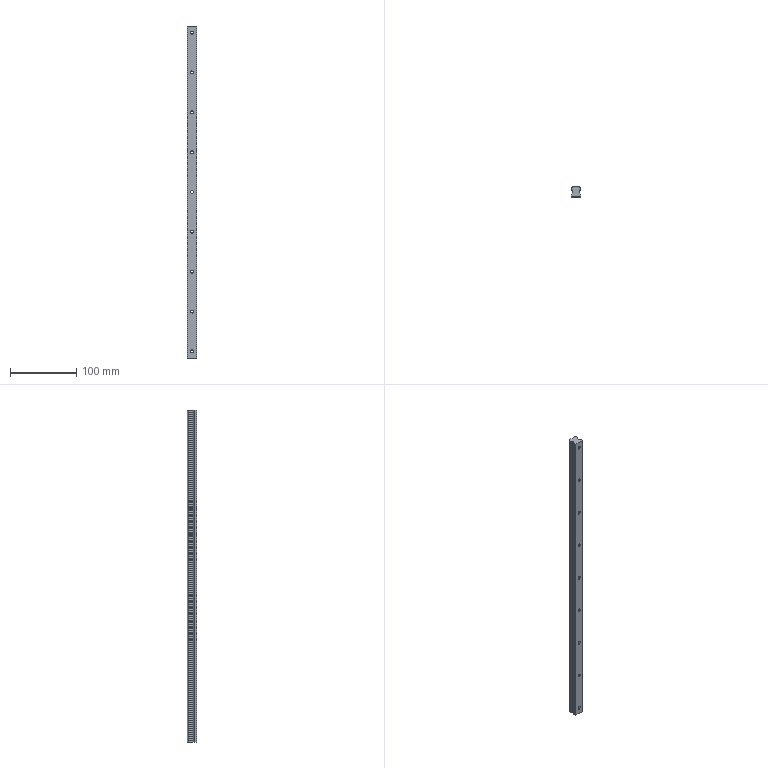Part | SolidWorks | features MirrorStock 1 | 1 solid | 81 faces | box 15 x 15 x 500 mm | volume 91810 mm3 | cylinder 50 | plane 31 | commonest cylinder face diameters 4.5 x18 8 x18 0.8 x8 3.24 x4 2 x2